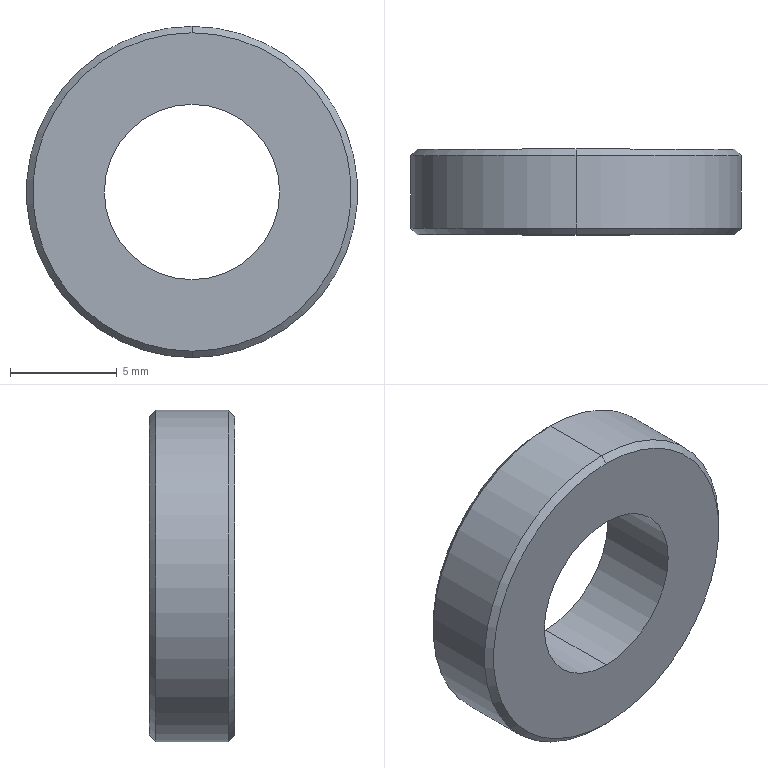Part | STEP file | 1 solid | 10 faces | box 15.5 x 4 x 15.5 mm | volume 539.201 mm3 | cone 4 | cylinder 4 | plane 2 | commonest cylinder face diameters 8.2 x2 15.5 x2
STEP:
#1=CARTESIAN_POINT('',(0.,0.,0.));
#2=DIRECTION('',(0.,0.,1.));
#3=DIRECTION('',(1.,0.,0.));
#4=AXIS2_PLACEMENT_3D('',#1,#2,#3);
#5=CARTESIAN_POINT('',(0.,4.,7.45));
#6=VERTEX_POINT('',#5);
#7=CARTESIAN_POINT('',(0.,4.,-7.45));
#8=VERTEX_POINT('',#7);
#9=CARTESIAN_POINT('',(0.,4.,0.));
#10=DIRECTION('',(0.,1.,0.));
#11=DIRECTION('',(0.,0.,1.));
#12=AXIS2_PLACEMENT_3D('',#9,#10,#11);
#13=CIRCLE('',#12,7.45);
#14=CARTESIAN_POINT('',(0.,4.,0.));
#15=DIRECTION('',(0.,-1.,0.));
#16=DIRECTION('',(0.,0.,-1.));
#17=AXIS2_PLACEMENT_3D('',#14,#15,#16);
#18=CONICAL_SURFACE('',#17,7.45,0.7854);
#19=CARTESIAN_POINT('',(3.142,0.));
#20=DIRECTION('',(-1.,0.));
#21=VECTOR('',#20,1.);
#22=LINE('',#19,#21);
#23=(GEOMETRIC_REPRESENTATION_CONTEXT(2)PARAMETRIC_REPRESENTATION_CONTEXT()REPRESENTATION_CONTEXT('',''));
#24=DEFINITIONAL_REPRESENTATION('',(#22),#23);
#25=PCURVE('',#18,#24);
#26=CARTESIAN_POINT('',(0.,4.,0.));
#27=DIRECTION('',(0.,1.,0.));
#28=DIRECTION('',(0.,0.,1.));
#29=AXIS2_PLACEMENT_3D('',#26,#27,#28);
#30=PLANE('',#29);
#31=CARTESIAN_POINT('',(0.,0.));
#32=DIRECTION('',(1.,0.));
#33=AXIS2_PLACEMENT_2D('',#31,#32);
#34=CIRCLE('',#33,7.45);
#35=(GEOMETRIC_REPRESENTATION_CONTEXT(2)PARAMETRIC_REPRESENTATION_CONTEXT()REPRESENTATION_CONTEXT('',''));
#36=DEFINITIONAL_REPRESENTATION('',(#34),#35);
#37=PCURVE('',#30,#36);
#38=SURFACE_CURVE('',#13,(#25,#37),.PCURVE_S1.);
#39=EDGE_CURVE('',#6,#8,#38,.T.);
#40=ORIENTED_EDGE('',*,*,#39,.F.);
#41=CARTESIAN_POINT('',(0.,3.7,7.75));
#42=VERTEX_POINT('',#41);
#43=CARTESIAN_POINT('',(0.,4.,7.45));
#44=DIRECTION('',(0.,-0.7071,0.7071));
#45=VECTOR('',#44,1.);
#46=LINE('',#43,#45);
#47=CARTESIAN_POINT('',(3.142,0.));
#48=DIRECTION('',(0.,1.));
#49=VECTOR('',#48,1.);
#50=LINE('',#47,#49);
#51=(GEOMETRIC_REPRESENTATION_CONTEXT(2)PARAMETRIC_REPRESENTATION_CONTEXT()REPRESENTATION_CONTEXT('',''));
#52=DEFINITIONAL_REPRESENTATION('',(#50),#51);
#53=PCURVE('',#18,#52);
#54=CARTESIAN_POINT('',(0.,4.,0.));
#55=DIRECTION('',(0.,-1.,0.));
#56=DIRECTION('',(0.,0.,-1.));
#57=AXIS2_PLACEMENT_3D('',#54,#55,#56);
#58=CONICAL_SURFACE('',#57,7.45,0.7854);
#59=CARTESIAN_POINT('',(3.142,0.));
#60=DIRECTION('',(0.,1.));
#61=VECTOR('',#60,1.);
#62=LINE('',#59,#61);
#63=(GEOMETRIC_REPRESENTATION_CONTEXT(2)PARAMETRIC_REPRESENTATION_CONTEXT()REPRESENTATION_CONTEXT('',''));
#64=DEFINITIONAL_REPRESENTATION('',(#62),#63);
#65=PCURVE('',#58,#64);
#66=SURFACE_CURVE('',#46,(#53,#65),.PCURVE_S1.);
#67=EDGE_CURVE('',#6,#42,#66,.T.);
#68=ORIENTED_EDGE('',*,*,#67,.T.);
#69=CARTESIAN_POINT('',(0.,3.7,-7.75));
#70=VERTEX_POINT('',#69);
#71=CARTESIAN_POINT('',(0.,3.7,0.));
#72=DIRECTION('',(0.,-1.,0.));
#73=DIRECTION('',(0.,0.,1.));
#74=AXIS2_PLACEMENT_3D('',#71,#72,#73);
#75=CIRCLE('',#74,7.75);
#76=CARTESIAN_POINT('',(-3.142,0.3));
#77=DIRECTION('',(1.,0.));
#78=VECTOR('',#77,1.);
#79=LINE('',#76,#78);
#80=(GEOMETRIC_REPRESENTATION_CONTEXT(2)PARAMETRIC_REPRESENTATION_CONTEXT()REPRESENTATION_CONTEXT('',''));
#81=DEFINITIONAL_REPRESENTATION('',(#79),#80);
#82=PCURVE('',#18,#81);
#83=CARTESIAN_POINT('',(0.,4.,0.));
#84=DIRECTION('',(0.,-1.,0.));
#85=DIRECTION('',(0.,0.,-1.));
#86=AXIS2_PLACEMENT_3D('',#83,#84,#85);
#87=CYLINDRICAL_SURFACE('',#86,7.75);
#88=CARTESIAN_POINT('',(-3.142,0.3));
#89=DIRECTION('',(1.,0.));
#90=VECTOR('',#89,1.);
#91=LINE('',#88,#90);
#92=(GEOMETRIC_REPRESENTATION_CONTEXT(2)PARAMETRIC_REPRESENTATION_CONTEXT()REPRESENTATION_CONTEXT('',''));
#93=DEFINITIONAL_REPRESENTATION('',(#91),#92);
#94=PCURVE('',#87,#93);
#95=SURFACE_CURVE('',#75,(#82,#94),.PCURVE_S1.);
#96=EDGE_CURVE('',#70,#42,#95,.T.);
#97=ORIENTED_EDGE('',*,*,#96,.F.);
#98=CARTESIAN_POINT('',(0.,4.,-7.45));
#99=DIRECTION('',(0.,-0.7071,-0.7071));
#100=VECTOR('',#99,1.);
#101=LINE('',#98,#100);
#102=CARTESIAN_POINT('',(0.,0.));
#103=DIRECTION('',(0.,1.));
#104=VECTOR('',#103,1.);
#105=LINE('',#102,#104);
#106=(GEOMETRIC_REPRESENTATION_CONTEXT(2)PARAMETRIC_REPRESENTATION_CONTEXT()REPRESENTATION_CONTEXT('',''));
#107=DEFINITIONAL_REPRESENTATION('',(#105),#106);
#108=PCURVE('',#18,#107);
#109=CARTESIAN_POINT('',(6.283,0.));
#110=DIRECTION('',(0.,1.));
#111=VECTOR('',#110,1.);
#112=LINE('',#109,#111);
#113=(GEOMETRIC_REPRESENTATION_CONTEXT(2)PARAMETRIC_REPRESENTATION_CONTEXT()REPRESENTATION_CONTEXT('',''));
#114=DEFINITIONAL_REPRESENTATION('',(#112),#113);
#115=PCURVE('',#58,#114);
#116=SURFACE_CURVE('',#101,(#108,#115),.PCURVE_S1.);
#117=EDGE_CURVE('',#8,#70,#116,.T.);
#118=ORIENTED_EDGE('',*,*,#117,.F.);
#119=EDGE_LOOP('',(#40,#68,#97,#118));
#120=FACE_BOUND('',#119,.T.);
#121=ADVANCED_FACE('',(#120),#18,.T.);
#122=CARTESIAN_POINT('',(0.,0.,-7.45));
#123=VERTEX_POINT('',#122);
#124=CARTESIAN_POINT('',(0.,0.,7.45));
#125=VERTEX_POINT('',#124);
#126=CARTESIAN_POINT('',(0.,0.,0.));
#127=DIRECTION('',(0.,-1.,0.));
#128=DIRECTION('',(0.,0.,1.));
#129=AXIS2_PLACEMENT_3D('',#126,#127,#128);
#130=CIRCLE('',#129,7.45);
#131=CARTESIAN_POINT('',(0.,0.3,0.));
#132=DIRECTION('',(0.,1.,0.));
#133=DIRECTION('',(0.,0.,1.));
#134=AXIS2_PLACEMENT_3D('',#131,#132,#133);
#135=CONICAL_SURFACE('',#134,7.75,0.7854);
#136=CARTESIAN_POINT('',(6.283,-0.3));
#137=DIRECTION('',(-1.,0.));
#138=VECTOR('',#137,1.);
#139=LINE('',#136,#138);
#140=(GEOMETRIC_REPRESENTATION_CONTEXT(2)PARAMETRIC_REPRESENTATION_CONTEXT()REPRESENTATION_CONTEXT('',''));
#141=DEFINITIONAL_REPRESENTATION('',(#139),#140);
#142=PCURVE('',#135,#141);
#143=CARTESIAN_POINT('',(0.,0.,0.));
#144=DIRECTION('',(0.,1.,0.));
#145=DIRECTION('',(0.,0.,1.));
#146=AXIS2_PLACEMENT_3D('',#143,#144,#145);
#147=PLANE('',#146);
#148=CARTESIAN_POINT('',(7.45,0.));
#149=CARTESIAN_POINT('',(7.45,-12.904));
#150=CARTESIAN_POINT('',(-3.725,-6.452));
#151=CARTESIAN_POINT('',(-14.9,0.));
#152=CARTESIAN_POINT('',(-3.725,6.452));
#153=CARTESIAN_POINT('',(7.45,12.904));
#154=CARTESIAN_POINT('',(7.45,0.));
#155=(BOUNDED_CURVE()B_SPLINE_CURVE(2,(#148,#149,#150,#151,#152,#153,#154),.UNSPECIFIED.,.T.,.F.)B_SPLINE_CURVE_WITH_KNOTS((1,2,2,2,2,1),(-2.094,0.,2.094,4.189,6.283,8.378),.UNSPECIFIED.)CURVE()GEOMETRIC_REPRESENTATION_ITEM()RATIONAL_B_SPLINE_CURVE((1.,0.5,1.,0.5,1.,0.5,1.))REPRESENTATION_ITEM(''));
#156=(GEOMETRIC_REPRESENTATION_CONTEXT(2)PARAMETRIC_REPRESENTATION_CONTEXT()REPRESENTATION_CONTEXT('',''));
#157=DEFINITIONAL_REPRESENTATION('',(#155),#156);
#158=PCURVE('',#147,#157);
#159=SURFACE_CURVE('',#130,(#142,#158),.PCURVE_S1.);
#160=EDGE_CURVE('',#123,#125,#159,.T.);
#161=ORIENTED_EDGE('',*,*,#160,.F.);
#162=CARTESIAN_POINT('',(0.,0.3,-7.75));
#163=VERTEX_POINT('',#162);
#164=CARTESIAN_POINT('',(0.,0.3,-7.75));
#165=DIRECTION('',(0.,0.7071,-0.7071));
#166=VECTOR('',#165,1.);
#167=LINE('',#164,#166);
#168=CARTESIAN_POINT('',(3.142,0.));
#169=DIRECTION('',(0.,1.));
#170=VECTOR('',#169,1.);
#171=LINE('',#168,#170);
#172=(GEOMETRIC_REPRESENTATION_CONTEXT(2)PARAMETRIC_REPRESENTATION_CONTEXT()REPRESENTATION_CONTEXT('',''));
#173=DEFINITIONAL_REPRESENTATION('',(#171),#172);
#174=PCURVE('',#135,#173);
#175=CARTESIAN_POINT('',(0.,0.3,0.));
#176=DIRECTION('',(0.,1.,0.));
#177=DIRECTION('',(0.,0.,1.));
#178=AXIS2_PLACEMENT_3D('',#175,#176,#177);
#179=CONICAL_SURFACE('',#178,7.75,0.7854);
#180=CARTESIAN_POINT('',(3.142,0.));
#181=DIRECTION('',(0.,1.));
#182=VECTOR('',#181,1.);
#183=LINE('',#180,#182);
#184=(GEOMETRIC_REPRESENTATION_CONTEXT(2)PARAMETRIC_REPRESENTATION_CONTEXT()REPRESENTATION_CONTEXT('',''));
#185=DEFINITIONAL_REPRESENTATION('',(#183),#184);
#186=PCURVE('',#179,#185);
#187=SURFACE_CURVE('',#167,(#174,#186),.PCURVE_S1.);
#188=EDGE_CURVE('',#123,#163,#187,.T.);
#189=ORIENTED_EDGE('',*,*,#188,.T.);
#190=CARTESIAN_POINT('',(0.,0.3,7.75));
#191=VERTEX_POINT('',#190);
#192=CARTESIAN_POINT('',(0.,0.3,0.));
#193=DIRECTION('',(0.,1.,0.));
#194=DIRECTION('',(0.,0.,1.));
#195=AXIS2_PLACEMENT_3D('',#192,#193,#194);
#196=CIRCLE('',#195,7.75);
#197=CARTESIAN_POINT('',(0.,0.));
#198=DIRECTION('',(1.,0.));
#199=VECTOR('',#198,1.);
#200=LINE('',#197,#199);
#201=(GEOMETRIC_REPRESENTATION_CONTEXT(2)PARAMETRIC_REPRESENTATION_CONTEXT()REPRESENTATION_CONTEXT('',''));
#202=DEFINITIONAL_REPRESENTATION('',(#200),#201);
#203=PCURVE('',#135,#202);
#204=CARTESIAN_POINT('',(3.142,3.7));
#205=DIRECTION('',(-1.,0.));
#206=VECTOR('',#205,1.);
#207=LINE('',#204,#206);
#208=(GEOMETRIC_REPRESENTATION_CONTEXT(2)PARAMETRIC_REPRESENTATION_CONTEXT()REPRESENTATION_CONTEXT('',''));
#209=DEFINITIONAL_REPRESENTATION('',(#207),#208);
#210=PCURVE('',#87,#209);
#211=SURFACE_CURVE('',#196,(#203,#210),.PCURVE_S1.);
#212=EDGE_CURVE('',#191,#163,#211,.T.);
#213=ORIENTED_EDGE('',*,*,#212,.F.);
#214=CARTESIAN_POINT('',(0.,0.3,7.75));
#215=DIRECTION('',(0.,0.7071,0.7071));
#216=VECTOR('',#215,1.);
#217=LINE('',#214,#216);
#218=CARTESIAN_POINT('',(0.,0.));
#219=DIRECTION('',(0.,1.));
#220=VECTOR('',#219,1.);
#221=LINE('',#218,#220);
#222=(GEOMETRIC_REPRESENTATION_CONTEXT(2)PARAMETRIC_REPRESENTATION_CONTEXT()REPRESENTATION_CONTEXT('',''));
#223=DEFINITIONAL_REPRESENTATION('',(#221),#222);
#224=PCURVE('',#135,#223);
#225=CARTESIAN_POINT('',(6.283,0.));
#226=DIRECTION('',(0.,1.));
#227=VECTOR('',#226,1.);
#228=LINE('',#225,#227);
#229=(GEOMETRIC_REPRESENTATION_CONTEXT(2)PARAMETRIC_REPRESENTATION_CONTEXT()REPRESENTATION_CONTEXT('',''));
#230=DEFINITIONAL_REPRESENTATION('',(#228),#229);
#231=PCURVE('',#179,#230);
#232=SURFACE_CURVE('',#217,(#224,#231),.PCURVE_S1.);
#233=EDGE_CURVE('',#125,#191,#232,.T.);
#234=ORIENTED_EDGE('',*,*,#233,.F.);
#235=EDGE_LOOP('',(#161,#189,#213,#234));
#236=FACE_BOUND('',#235,.T.);
#237=ADVANCED_FACE('',(#236),#135,.T.);
#238=CARTESIAN_POINT('',(0.,4.,-4.1));
#239=VERTEX_POINT('',#238);
#240=CARTESIAN_POINT('',(0.,0.,-4.1));
#241=VERTEX_POINT('',#240);
#242=CARTESIAN_POINT('',(0.,4.,-4.1));
#243=DIRECTION('',(0.,-1.,0.));
#244=VECTOR('',#243,1.);
#245=LINE('',#242,#244);
#246=CARTESIAN_POINT('',(0.,4.,0.));
#247=DIRECTION('',(0.,-1.,0.));
#248=DIRECTION('',(0.,0.,-1.));
#249=AXIS2_PLACEMENT_3D('',#246,#247,#248);
#250=CYLINDRICAL_SURFACE('',#249,4.1);
#251=CARTESIAN_POINT('',(6.283,0.));
#252=DIRECTION('',(0.,1.));
#253=VECTOR('',#252,1.);
#254=LINE('',#251,#253);
#255=(GEOMETRIC_REPRESENTATION_CONTEXT(2)PARAMETRIC_REPRESENTATION_CONTEXT()REPRESENTATION_CONTEXT('',''));
#256=DEFINITIONAL_REPRESENTATION('',(#254),#255);
#257=PCURVE('',#250,#256);
#258=CARTESIAN_POINT('',(0.,4.,0.));
#259=DIRECTION('',(0.,-1.,0.));
#260=DIRECTION('',(0.,0.,-1.));
#261=AXIS2_PLACEMENT_3D('',#258,#259,#260);
#262=CYLINDRICAL_SURFACE('',#261,4.1);
#263=CARTESIAN_POINT('',(0.,0.));
#264=DIRECTION('',(0.,1.));
#265=VECTOR('',#264,1.);
#266=LINE('',#263,#265);
#267=(GEOMETRIC_REPRESENTATION_CONTEXT(2)PARAMETRIC_REPRESENTATION_CONTEXT()REPRESENTATION_CONTEXT('',''));
#268=DEFINITIONAL_REPRESENTATION('',(#266),#267);
#269=PCURVE('',#262,#268);
#270=SURFACE_CURVE('',#245,(#257,#269),.PCURVE_S1.);
#271=EDGE_CURVE('',#239,#241,#270,.T.);
#272=ORIENTED_EDGE('',*,*,#271,.T.);
#273=CARTESIAN_POINT('',(0.,0.,4.1));
#274=VERTEX_POINT('',#273);
#275=CARTESIAN_POINT('',(0.,0.,0.));
#276=DIRECTION('',(0.,1.,0.));
#277=DIRECTION('',(0.,0.,1.));
#278=AXIS2_PLACEMENT_3D('',#275,#276,#277);
#279=CIRCLE('',#278,4.1);
#280=CARTESIAN_POINT('',(9.425,4.));
#281=DIRECTION('',(-1.,0.));
#282=VECTOR('',#281,1.);
#283=LINE('',#280,#282);
#284=(GEOMETRIC_REPRESENTATION_CONTEXT(2)PARAMETRIC_REPRESENTATION_CONTEXT()REPRESENTATION_CONTEXT('',''));
#285=DEFINITIONAL_REPRESENTATION('',(#283),#284);
#286=PCURVE('',#250,#285);
#287=CARTESIAN_POINT('',(0.,0.));
#288=DIRECTION('',(1.,0.));
#289=AXIS2_PLACEMENT_2D('',#287,#288);
#290=CIRCLE('',#289,4.1);
#291=(GEOMETRIC_REPRESENTATION_CONTEXT(2)PARAMETRIC_REPRESENTATION_CONTEXT()REPRESENTATION_CONTEXT('',''));
#292=DEFINITIONAL_REPRESENTATION('',(#290),#291);
#293=PCURVE('',#147,#292);
#294=SURFACE_CURVE('',#279,(#286,#293),.PCURVE_S1.);
#295=EDGE_CURVE('',#241,#274,#294,.T.);
#296=ORIENTED_EDGE('',*,*,#295,.T.);
#297=CARTESIAN_POINT('',(0.,4.,4.1));
#298=VERTEX_POINT('',#297);
#299=CARTESIAN_POINT('',(0.,4.,4.1));
#300=DIRECTION('',(0.,-1.,0.));
#301=VECTOR('',#300,1.);
#302=LINE('',#299,#301);
#303=CARTESIAN_POINT('',(3.142,0.));
#304=DIRECTION('',(0.,1.));
#305=VECTOR('',#304,1.);
#306=LINE('',#303,#305);
#307=(GEOMETRIC_REPRESENTATION_CONTEXT(2)PARAMETRIC_REPRESENTATION_CONTEXT()REPRESENTATION_CONTEXT('',''));
#308=DEFINITIONAL_REPRESENTATION('',(#306),#307);
#309=PCURVE('',#250,#308);
#310=CARTESIAN_POINT('',(3.142,0.));
#311=DIRECTION('',(0.,1.));
#312=VECTOR('',#311,1.);
#313=LINE('',#310,#312);
#314=(GEOMETRIC_REPRESENTATION_CONTEXT(2)PARAMETRIC_REPRESENTATION_CONTEXT()REPRESENTATION_CONTEXT('',''));
#315=DEFINITIONAL_REPRESENTATION('',(#313),#314);
#316=PCURVE('',#262,#315);
#317=SURFACE_CURVE('',#302,(#309,#316),.PCURVE_S1.);
#318=EDGE_CURVE('',#298,#274,#317,.T.);
#319=ORIENTED_EDGE('',*,*,#318,.F.);
#320=CARTESIAN_POINT('',(0.,4.,0.));
#321=DIRECTION('',(0.,1.,0.));
#322=DIRECTION('',(0.,0.,1.));
#323=AXIS2_PLACEMENT_3D('',#320,#321,#322);
#324=CIRCLE('',#323,4.1);
#325=CARTESIAN_POINT('',(9.425,0.));
#326=DIRECTION('',(-1.,0.));
#327=VECTOR('',#326,1.);
#328=LINE('',#325,#327);
#329=(GEOMETRIC_REPRESENTATION_CONTEXT(2)PARAMETRIC_REPRESENTATION_CONTEXT()REPRESENTATION_CONTEXT('',''));
#330=DEFINITIONAL_REPRESENTATION('',(#328),#329);
#331=PCURVE('',#250,#330);
#332=CARTESIAN_POINT('',(0.,0.));
#333=DIRECTION('',(1.,0.));
#334=AXIS2_PLACEMENT_2D('',#332,#333);
#335=CIRCLE('',#334,4.1);
#336=(GEOMETRIC_REPRESENTATION_CONTEXT(2)PARAMETRIC_REPRESENTATION_CONTEXT()REPRESENTATION_CONTEXT('',''));
#337=DEFINITIONAL_REPRESENTATION('',(#335),#336);
#338=PCURVE('',#30,#337);
#339=SURFACE_CURVE('',#324,(#331,#338),.PCURVE_S1.);
#340=EDGE_CURVE('',#239,#298,#339,.T.);
#341=ORIENTED_EDGE('',*,*,#340,.F.);
#342=EDGE_LOOP('',(#272,#296,#319,#341));
#343=FACE_BOUND('',#342,.F.);
#344=ADVANCED_FACE('',(#343),#250,.F.);
#345=ORIENTED_EDGE('',*,*,#96,.T.);
#346=CARTESIAN_POINT('',(0.,4.,7.75));
#347=DIRECTION('',(0.,-1.,0.));
#348=VECTOR('',#347,1.);
#349=LINE('',#346,#348);
#350=CARTESIAN_POINT('',(3.142,0.));
#351=DIRECTION('',(0.,1.));
#352=VECTOR('',#351,1.);
#353=LINE('',#350,#352);
#354=(GEOMETRIC_REPRESENTATION_CONTEXT(2)PARAMETRIC_REPRESENTATION_CONTEXT()REPRESENTATION_CONTEXT('',''));
#355=DEFINITIONAL_REPRESENTATION('',(#353),#354);
#356=PCURVE('',#87,#355);
#357=CARTESIAN_POINT('',(0.,4.,0.));
#358=DIRECTION('',(0.,-1.,0.));
#359=DIRECTION('',(0.,0.,-1.));
#360=AXIS2_PLACEMENT_3D('',#357,#358,#359);
#361=CYLINDRICAL_SURFACE('',#360,7.75);
#362=CARTESIAN_POINT('',(3.142,0.));
#363=DIRECTION('',(0.,1.));
#364=VECTOR('',#363,1.);
#365=LINE('',#362,#364);
#366=(GEOMETRIC_REPRESENTATION_CONTEXT(2)PARAMETRIC_REPRESENTATION_CONTEXT()REPRESENTATION_CONTEXT('',''));
#367=DEFINITIONAL_REPRESENTATION('',(#365),#366);
#368=PCURVE('',#361,#367);
#369=SURFACE_CURVE('',#349,(#356,#368),.PCURVE_S1.);
#370=EDGE_CURVE('',#42,#191,#369,.T.);
#371=ORIENTED_EDGE('',*,*,#370,.T.);
#372=ORIENTED_EDGE('',*,*,#212,.T.);
#373=CARTESIAN_POINT('',(0.,4.,-7.75));
#374=DIRECTION('',(0.,-1.,0.));
#375=VECTOR('',#374,1.);
#376=LINE('',#373,#375);
#377=CARTESIAN_POINT('',(0.,0.));
#378=DIRECTION('',(0.,1.));
#379=VECTOR('',#378,1.);
#380=LINE('',#377,#379);
#381=(GEOMETRIC_REPRESENTATION_CONTEXT(2)PARAMETRIC_REPRESENTATION_CONTEXT()REPRESENTATION_CONTEXT('',''));
#382=DEFINITIONAL_REPRESENTATION('',(#380),#381);
#383=PCURVE('',#87,#382);
#384=CARTESIAN_POINT('',(6.283,0.));
#385=DIRECTION('',(0.,1.));
#386=VECTOR('',#385,1.);
#387=LINE('',#384,#386);
#388=(GEOMETRIC_REPRESENTATION_CONTEXT(2)PARAMETRIC_REPRESENTATION_CONTEXT()REPRESENTATION_CONTEXT('',''));
#389=DEFINITIONAL_REPRESENTATION('',(#387),#388);
#390=PCURVE('',#361,#389);
#391=SURFACE_CURVE('',#376,(#383,#390),.PCURVE_S1.);
#392=EDGE_CURVE('',#70,#163,#391,.T.);
#393=ORIENTED_EDGE('',*,*,#392,.F.);
#394=EDGE_LOOP('',(#345,#371,#372,#393));
#395=FACE_BOUND('',#394,.T.);
#396=ADVANCED_FACE('',(#395),#87,.T.);
#397=CARTESIAN_POINT('',(0.,4.,0.));
#398=DIRECTION('',(0.,1.,0.));
#399=DIRECTION('',(0.,0.,1.));
#400=AXIS2_PLACEMENT_3D('',#397,#398,#399);
#401=CIRCLE('',#400,7.45);
#402=CARTESIAN_POINT('',(0.,0.));
#403=DIRECTION('',(1.,0.));
#404=AXIS2_PLACEMENT_2D('',#402,#403);
#405=CIRCLE('',#404,7.45);
#406=(GEOMETRIC_REPRESENTATION_CONTEXT(2)PARAMETRIC_REPRESENTATION_CONTEXT()REPRESENTATION_CONTEXT('',''));
#407=DEFINITIONAL_REPRESENTATION('',(#405),#406);
#408=PCURVE('',#30,#407);
#409=CARTESIAN_POINT('',(9.425,0.));
#410=DIRECTION('',(-1.,0.));
#411=VECTOR('',#410,1.);
#412=LINE('',#409,#411);
#413=(GEOMETRIC_REPRESENTATION_CONTEXT(2)PARAMETRIC_REPRESENTATION_CONTEXT()REPRESENTATION_CONTEXT('',''));
#414=DEFINITIONAL_REPRESENTATION('',(#412),#413);
#415=PCURVE('',#58,#414);
#416=SURFACE_CURVE('',#401,(#408,#415),.PCURVE_S1.);
#417=EDGE_CURVE('',#8,#6,#416,.T.);
#418=ORIENTED_EDGE('',*,*,#417,.T.);
#419=ORIENTED_EDGE('',*,*,#39,.T.);
#420=EDGE_LOOP('',(#418,#419));
#421=FACE_BOUND('',#420,.T.);
#422=ORIENTED_EDGE('',*,*,#340,.F.);
#423=CARTESIAN_POINT('',(0.,4.,0.));
#424=DIRECTION('',(0.,1.,0.));
#425=DIRECTION('',(0.,0.,1.));
#426=AXIS2_PLACEMENT_3D('',#423,#424,#425);
#427=CIRCLE('',#426,4.1);
#428=CARTESIAN_POINT('',(0.,0.));
#429=DIRECTION('',(1.,0.));
#430=AXIS2_PLACEMENT_2D('',#428,#429);
#431=CIRCLE('',#430,4.1);
#432=(GEOMETRIC_REPRESENTATION_CONTEXT(2)PARAMETRIC_REPRESENTATION_CONTEXT()REPRESENTATION_CONTEXT('',''));
#433=DEFINITIONAL_REPRESENTATION('',(#431),#432);
#434=PCURVE('',#30,#433);
#435=CARTESIAN_POINT('',(3.142,0.));
#436=DIRECTION('',(-1.,0.));
#437=VECTOR('',#436,1.);
#438=LINE('',#435,#437);
#439=(GEOMETRIC_REPRESENTATION_CONTEXT(2)PARAMETRIC_REPRESENTATION_CONTEXT()REPRESENTATION_CONTEXT('',''));
#440=DEFINITIONAL_REPRESENTATION('',(#438),#439);
#441=PCURVE('',#262,#440);
#442=SURFACE_CURVE('',#427,(#434,#441),.PCURVE_S1.);
#443=EDGE_CURVE('',#298,#239,#442,.T.);
#444=ORIENTED_EDGE('',*,*,#443,.F.);
#445=EDGE_LOOP('',(#422,#444));
#446=FACE_BOUND('',#445,.T.);
#447=ADVANCED_FACE('',(#421,#446),#30,.T.);
#448=CARTESIAN_POINT('',(0.,0.,0.));
#449=DIRECTION('',(0.,-1.,0.));
#450=DIRECTION('',(0.,0.,1.));
#451=AXIS2_PLACEMENT_3D('',#448,#449,#450);
#452=CIRCLE('',#451,7.45);
#453=CARTESIAN_POINT('',(7.45,0.));
#454=CARTESIAN_POINT('',(7.45,-12.904));
#455=CARTESIAN_POINT('',(-3.725,-6.452));
#456=CARTESIAN_POINT('',(-14.9,0.));
#457=CARTESIAN_POINT('',(-3.725,6.452));
#458=CARTESIAN_POINT('',(7.45,12.904));
#459=CARTESIAN_POINT('',(7.45,0.));
#460=(BOUNDED_CURVE()B_SPLINE_CURVE(2,(#453,#454,#455,#456,#457,#458,#459),.UNSPECIFIED.,.T.,.F.)B_SPLINE_CURVE_WITH_KNOTS((1,2,2,2,2,1),(-2.094,0.,2.094,4.189,6.283,8.378),.UNSPECIFIED.)CURVE()GEOMETRIC_REPRESENTATION_ITEM()RATIONAL_B_SPLINE_CURVE((1.,0.5,1.,0.5,1.,0.5,1.))REPRESENTATION_ITEM(''));
#461=(GEOMETRIC_REPRESENTATION_CONTEXT(2)PARAMETRIC_REPRESENTATION_CONTEXT()REPRESENTATION_CONTEXT('',''));
#462=DEFINITIONAL_REPRESENTATION('',(#460),#461);
#463=PCURVE('',#147,#462);
#464=CARTESIAN_POINT('',(6.283,-0.3));
#465=DIRECTION('',(-1.,0.));
#466=VECTOR('',#465,1.);
#467=LINE('',#464,#466);
#468=(GEOMETRIC_REPRESENTATION_CONTEXT(2)PARAMETRIC_REPRESENTATION_CONTEXT()REPRESENTATION_CONTEXT('',''));
#469=DEFINITIONAL_REPRESENTATION('',(#467),#468);
#470=PCURVE('',#179,#469);
#471=SURFACE_CURVE('',#452,(#463,#470),.PCURVE_S1.);
#472=EDGE_CURVE('',#125,#123,#471,.T.);
#473=ORIENTED_EDGE('',*,*,#472,.T.);
#474=ORIENTED_EDGE('',*,*,#160,.T.);
#475=EDGE_LOOP('',(#473,#474));
#476=FACE_BOUND('',#475,.T.);
#477=ORIENTED_EDGE('',*,*,#295,.T.);
#478=CARTESIAN_POINT('',(0.,0.,0.));
#479=DIRECTION('',(0.,1.,0.));
#480=DIRECTION('',(0.,0.,1.));
#481=AXIS2_PLACEMENT_3D('',#478,#479,#480);
#482=CIRCLE('',#481,4.1);
#483=CARTESIAN_POINT('',(0.,0.));
#484=DIRECTION('',(1.,0.));
#485=AXIS2_PLACEMENT_2D('',#483,#484);
#486=CIRCLE('',#485,4.1);
#487=(GEOMETRIC_REPRESENTATION_CONTEXT(2)PARAMETRIC_REPRESENTATION_CONTEXT()REPRESENTATION_CONTEXT('',''));
#488=DEFINITIONAL_REPRESENTATION('',(#486),#487);
#489=PCURVE('',#147,#488);
#490=CARTESIAN_POINT('',(3.142,4.));
#491=DIRECTION('',(-1.,0.));
#492=VECTOR('',#491,1.);
#493=LINE('',#490,#492);
#494=(GEOMETRIC_REPRESENTATION_CONTEXT(2)PARAMETRIC_REPRESENTATION_CONTEXT()REPRESENTATION_CONTEXT('',''));
#495=DEFINITIONAL_REPRESENTATION('',(#493),#494);
#496=PCURVE('',#262,#495);
#497=SURFACE_CURVE('',#482,(#489,#496),.PCURVE_S1.);
#498=EDGE_CURVE('',#274,#241,#497,.T.);
#499=ORIENTED_EDGE('',*,*,#498,.T.);
#500=EDGE_LOOP('',(#477,#499));
#501=FACE_BOUND('',#500,.T.);
#502=ADVANCED_FACE('',(#476,#501),#147,.F.);
#503=ORIENTED_EDGE('',*,*,#370,.F.);
#504=CARTESIAN_POINT('',(0.,3.7,0.));
#505=DIRECTION('',(0.,-1.,0.));
#506=DIRECTION('',(0.,0.,1.));
#507=AXIS2_PLACEMENT_3D('',#504,#505,#506);
#508=CIRCLE('',#507,7.75);
#509=CARTESIAN_POINT('',(3.142,0.3));
#510=DIRECTION('',(1.,0.));
#511=VECTOR('',#510,1.);
#512=LINE('',#509,#511);
#513=(GEOMETRIC_REPRESENTATION_CONTEXT(2)PARAMETRIC_REPRESENTATION_CONTEXT()REPRESENTATION_CONTEXT('',''));
#514=DEFINITIONAL_REPRESENTATION('',(#512),#513);
#515=PCURVE('',#361,#514);
#516=CARTESIAN_POINT('',(3.142,0.3));
#517=DIRECTION('',(1.,0.));
#518=VECTOR('',#517,1.);
#519=LINE('',#516,#518);
#520=(GEOMETRIC_REPRESENTATION_CONTEXT(2)PARAMETRIC_REPRESENTATION_CONTEXT()REPRESENTATION_CONTEXT('',''));
#521=DEFINITIONAL_REPRESENTATION('',(#519),#520);
#522=PCURVE('',#58,#521);
#523=SURFACE_CURVE('',#508,(#515,#522),.PCURVE_S1.);
#524=EDGE_CURVE('',#42,#70,#523,.T.);
#525=ORIENTED_EDGE('',*,*,#524,.T.);
#526=ORIENTED_EDGE('',*,*,#392,.T.);
#527=CARTESIAN_POINT('',(0.,0.3,0.));
#528=DIRECTION('',(0.,1.,0.));
#529=DIRECTION('',(0.,0.,1.));
#530=AXIS2_PLACEMENT_3D('',#527,#528,#529);
#531=CIRCLE('',#530,7.75);
#532=CARTESIAN_POINT('',(9.425,3.7));
#533=DIRECTION('',(-1.,0.));
#534=VECTOR('',#533,1.);
#535=LINE('',#532,#534);
#536=(GEOMETRIC_REPRESENTATION_CONTEXT(2)PARAMETRIC_REPRESENTATION_CONTEXT()REPRESENTATION_CONTEXT('',''));
#537=DEFINITIONAL_REPRESENTATION('',(#535),#536);
#538=PCURVE('',#361,#537);
#539=CARTESIAN_POINT('',(0.,0.));
#540=DIRECTION('',(1.,0.));
#541=VECTOR('',#540,1.);
#542=LINE('',#539,#541);
#543=(GEOMETRIC_REPRESENTATION_CONTEXT(2)PARAMETRIC_REPRESENTATION_CONTEXT()REPRESENTATION_CONTEXT('',''));
#544=DEFINITIONAL_REPRESENTATION('',(#542),#543);
#545=PCURVE('',#179,#544);
#546=SURFACE_CURVE('',#531,(#538,#545),.PCURVE_S1.);
#547=EDGE_CURVE('',#163,#191,#546,.T.);
#548=ORIENTED_EDGE('',*,*,#547,.T.);
#549=EDGE_LOOP('',(#503,#525,#526,#548));
#550=FACE_BOUND('',#549,.T.);
#551=ADVANCED_FACE('',(#550),#361,.T.);
#552=ORIENTED_EDGE('',*,*,#498,.T.);
#553=ORIENTED_EDGE('',*,*,#271,.F.);
#554=ORIENTED_EDGE('',*,*,#443,.F.);
#555=ORIENTED_EDGE('',*,*,#318,.T.);
#556=EDGE_LOOP('',(#552,#553,#554,#555));
#557=FACE_BOUND('',#556,.F.);
#558=ADVANCED_FACE('',(#557),#262,.F.);
#559=ORIENTED_EDGE('',*,*,#188,.F.);
#560=ORIENTED_EDGE('',*,*,#472,.F.);
#561=ORIENTED_EDGE('',*,*,#233,.T.);
#562=ORIENTED_EDGE('',*,*,#547,.F.);
#563=EDGE_LOOP('',(#559,#560,#561,#562));
#564=FACE_BOUND('',#563,.T.);
#565=ADVANCED_FACE('',(#564),#179,.T.);
#566=ORIENTED_EDGE('',*,*,#67,.F.);
#567=ORIENTED_EDGE('',*,*,#417,.F.);
#568=ORIENTED_EDGE('',*,*,#117,.T.);
#569=ORIENTED_EDGE('',*,*,#524,.F.);
#570=EDGE_LOOP('',(#566,#567,#568,#569));
#571=FACE_BOUND('',#570,.T.);
#572=ADVANCED_FACE('',(#571),#58,.T.);
#573=CLOSED_SHELL('',(#121,#237,#344,#396,#447,#502,#551,#558,#565,#572));
#574=MANIFOLD_SOLID_BREP('',#573);
#575=(LENGTH_UNIT()NAMED_UNIT(*)SI_UNIT(.MILLI.,.METRE.));
#576=UNCERTAINTY_MEASURE_WITH_UNIT(LENGTH_MEASURE(0.0000001),#575,'','');
#577=(NAMED_UNIT(*)PLANE_ANGLE_UNIT()SI_UNIT($,.RADIAN.));
#578=(NAMED_UNIT(*)SI_UNIT($,.STERADIAN.)SOLID_ANGLE_UNIT());
#579=(GEOMETRIC_REPRESENTATION_CONTEXT(3)GLOBAL_UNCERTAINTY_ASSIGNED_CONTEXT((#576))GLOBAL_UNIT_ASSIGNED_CONTEXT((#575,#577,#578))REPRESENTATION_CONTEXT('',''));
#580=ADVANCED_BREP_SHAPE_REPRESENTATION('',(#4,#574),#579);